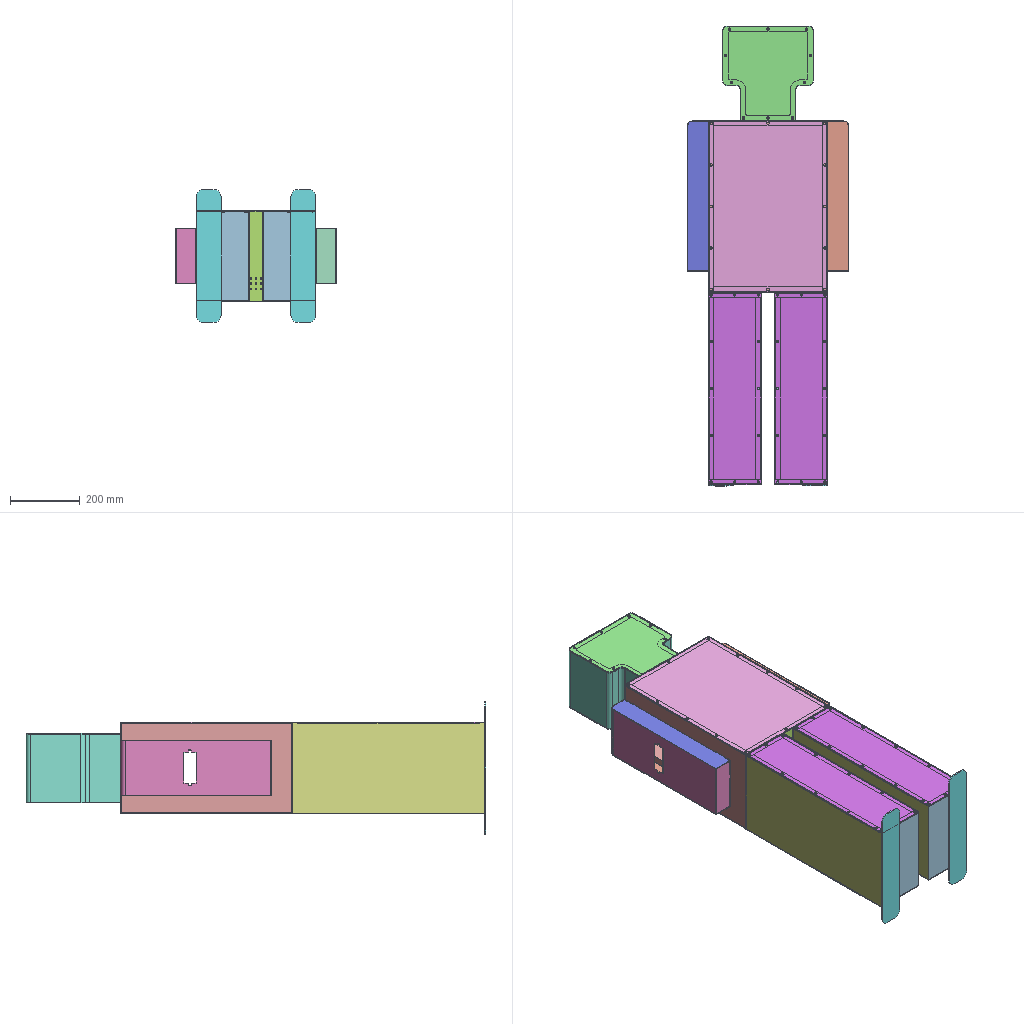Assembly | SolidWorks | 23 different items | 65 placed | box 460 x 1314 x 380 mm
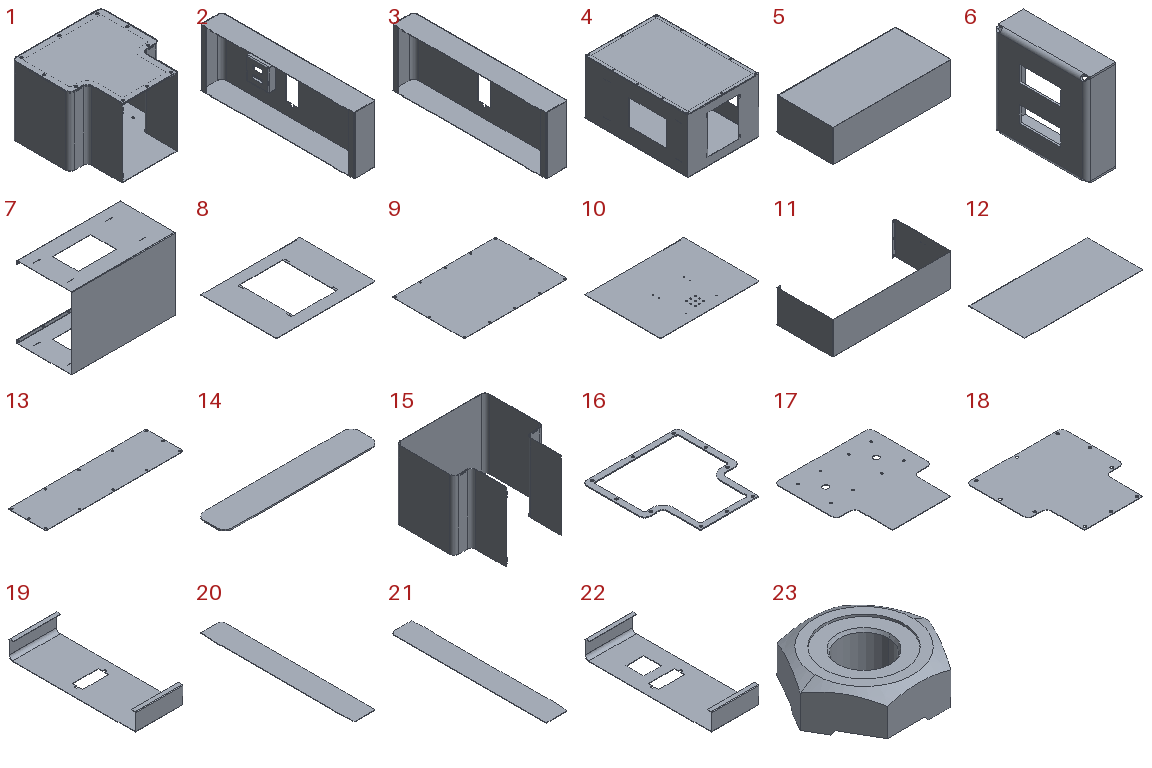Parts list (item | name | quantity | parent item | size | volume | features):
1 | (subassembly) | x1 | - | 260 x 272 x 200 mm | 384114 mm3 | -
2 | (subassembly) | x1 | - | 61.2 x 430 x 160 mm | 170255 mm3 | -
3 | (subassembly) | x1 | - | 61.2 x 430 x 160 mm | 165436 mm3 | -
4 | (subassembly) | x1 | - | 340 x 490 x 261.2 mm | 851284 mm3 | -
5 | (subassembly) | x2 | - | 550 x 261.2 x 150 mm | 653349 mm3 | features MirrorCompFeat 1, ReferencePattern 1
6 | - | x1 | in 2 | 20 x 62.4 x 62.4 mm | 9139 mm3 | features BaseBody 1
7 | - | x1 | in 4 | 487.6 x 260 x 340 mm | 463191 mm3 | features ICE 2, Cut 1, FlatPattern 1, MirrorPattern 1, SMBaseFlange 1, SheetMetal 1
8 | - | x1 | in 4 | 340 x 260 x 15 mm | 78192 mm3 | features Cut 2, EdgeFlange 1, FlatPattern 1, ICE 1, SMBaseFlange 1, SheetMetal 1
9 | - | x1 | in 4 | 490 x 340 x 1.2 mm | 199340 mm3 | features FlatPattern 1, SMBaseFlange 1, SheetMetal 1
10 | - | x1 | in 4 | 340 x 260 x 15 mm | 110561 mm3 | features ICE 2, EdgeFlange 1, FlatPattern 1, SMBaseFlange 1, SheetMetal 1
11 | - | x2 | in 5 | 550 x 260 x 150 mm | 196185 mm3 | features Cut 1, FlatPattern 1, ICE 1, SMBaseFlange 1, SheetMetal 1
12 | - | x4 | in 5 | 547.6 x 258.8 x 15 mm | 177930 mm3 | features EdgeFlange 1, FlatPattern 1, ICE 1, SMBaseFlange 1, SheetMetal 1
13 | - | x2 | in 5 | 550 x 150 x 1.2 mm | 98420 mm3 | features FlatPattern 1, SMBaseFlange 1, SheetMetal 1
14 | - | x2 | - | 380 x 70 x 3.2 mm | 84021 mm3 | features FlatPattern 1, SMBaseFlange 1, SheetMetal 1
15 | - | x1 | in 1 | 260 x 272 x 200 mm | 208024 mm3 | features ICE 2, SMBaseFlange 2, FlatPattern 1, MirrorPattern 1, SheetMetal 1
16 | - | x1 | in 1 | 257.6 x 269.6 x 2.3 mm | 32681 mm3 | features SMBaseFlange 2, FlatPattern 1, ICE 1, SheetMetal 1
17 | - | x1 | in 1 | 257.6 x 269.6 x 1.2 mm | 70428 mm3 | features HoleWzd 2, FlatPattern 1, SMBaseFlange 1, SheetMetal 1
18 | - | x1 | in 1 | 257.6 x 269.6 x 1.2 mm | 70578 mm3 | features FlatPattern 1, SMBaseFlange 1, SheetMetal 1
19 | - | x1 | in 3 | 160 x 430 x 60 mm | 105063 mm3 | features FlatPattern 1, ICE 1, SMBaseFlange 1, SheetMetal 1
20 | - | x2 | in 2, 3 | 60 x 427.6 x 1.2 mm | 30186 mm3 | features EdgeFlange 1, FlatPattern 1, SMBaseFlange 1, SheetMetal 1
21 | - | x2 | in 2, 3 | 60 x 427.6 x 1.2 mm | 30186 mm3 | features EdgeFlange 1, FlatPattern 1, SMBaseFlange 1, SheetMetal 1
22 | - | x1 | in 2 | 160 x 430 x 60 mm | 100743 mm3 | features FlatPattern 1, ICE 1, SMBaseFlange 1, SheetMetal 1
23 | - | x34 | in 1, 5 | 11.547 x 10 x 4 mm | 240.353 mm3 | features Cut 2, RevCut 2, Boss 1, Chamfer 1, CirPattern 1, Draft 1, Extrusion 1, LPattern 1, RefAxis 1
Mates (type | each side: item.copy, entity, surface, feature):
In the top assembly
Coincident | 8.1 face plane Base-Flange1 | 15.1 face plane Base-Flange1
DistanceDim | 7.1 face plane Base-Flange1 | 17.1 face plane Base-Flange1
DistanceDim | 15.1 face plane Base-Flange1 | 7.1 face plane Base-Flange1
Coincident | 10.1 face plane Base-Flange1 | 11.1 face plane Base-Flange1
Coincident | 7.1 face plane Base-Flange1 | 12.1 face plane Base-Flange1
Coincident | 7.1 face plane Base-Flange1 | 11.1 face plane Base-Flange1
Coincident | 10.1 face plane Base-Flange1 | 11.2 face plane Base-Flange1
Coincident | 7.1 face plane Base-Flange1 | 11.2 face plane Base-Flange1
Coincident | 7.1 face plane Base-Flange1 | 12.2 face plane Base-Flange1
Coincident | 7.1 face plane Base-Flange1 | 22.1 edge
Coincident | 8.1 face plane Base-Flange1 | 22.1 face plane Base-Flange1
DistanceDim | 7.1 face plane Base-Flange1 | 21.1 face plane Base-Flange1
Coincident | 7.1 face plane Base-Flange1 | 19.1 edge
Coincident | 8.1 face plane Base-Flange1 | 19.1 face plane Base-Flange1
DistanceDim | 7.1 face plane Base-Flange1 | 20.1 face plane Base-Flange1
Coincident | 11.2 face plane Base-Flange1 | 14.1 face plane Base-Flange1
Coincident | 12.2 face plane Base-Flange1 | 14.1 face plane Base-Flange1
DistanceDim | 11.2 face plane Base-Flange1 | 14.1 face plane Base-Flange1
In subassembly 2
InPlace | 22.2 face plane Base-Flange1 | 20.2 plane
InPlace | 22.2 face plane Base-Flange1 | 21.2 plane
Coincident | 22.2 face plane Base-Flange1 | 6.1 face plane Input1
Coincident | 22.2 face plane Cut-Extrude1 | 6.1 face plane Input1 | 2 times
In subassembly 3
InPlace | 19.2 face plane Base-Flange1 | 20.2 plane
InPlace | 19.2 face plane Base-Flange1 | 21.2 plane
In subassembly 5
InPlace | 11.3 face plane Base-Flange1 | 12.3 plane
InPlace | 12.3 face plane Edge-Flange1 | 13.1 plane
Concentric | 12.3 face cylinder Cut-Extrude1 | 23.1 face cylinder Cut-Extrude1
Coincident | 12.3 face plane Edge-Flange1 | 23.1 face plane BaseNut
Concentric | 12.3 face cylinder Cut-Extrude1 | 23.2 face cylinder Cut-Extrude1
Coincident | 12.3 face plane Edge-Flange1 | 23.2 face plane BaseNut
Concentric | 12.3 face cylinder Cut-Extrude1 | 23.3 face cylinder Cut-Extrude1
Coincident | 12.3 face plane Edge-Flange1 | 23.3 face plane BaseNut
Concentric | 12.4 face cylinder Cut-Extrude1 | 23.4 face cylinder Cut-Extrude1
Coincident | 12.4 face plane Edge-Flange1 | 23.4 face plane BaseNut
Concentric | 12.4 face cylinder Cut-Extrude1 | 23.5 face cylinder Cut-Extrude1
Coincident | 12.4 face plane Edge-Flange1 | 23.5 face plane BaseNut
Concentric | 12.4 face cylinder Cut-Extrude1 | 23.6 face cylinder Cut-Extrude1
Coincident | 12.4 face plane Edge-Flange1 | 23.6 face plane BaseNut
Concentric | 11.3 face cylinder Cut-Extrude1 | 23.7 face cylinder Cut-Extrude1
Coincident | 11.3 face plane Base-Flange1 | 23.7 face plane BaseNut
Concentric | 11.3 face cylinder Cut-Extrude1 | 23.8 face cylinder Cut-Extrude1
Coincident | 11.3 face plane Base-Flange1 | 23.8 face plane BaseNut
Concentric | 11.3 face cylinder Cut-Extrude1 | 23.9 face cylinder Cut-Extrude1
Coincident | 11.3 face plane Base-Flange1 | 23.9 face plane BaseNut
Concentric | 11.3 face cylinder Cut-Extrude1 | 23.10 face cylinder Cut-Extrude1
Coincident | 11.3 face plane Base-Flange1 | 23.10 face plane BaseNut
Concentric | 11.3 face cylinder Cut-Extrude1 | 23.11 face cylinder Cut-Extrude1
Coincident | 11.3 face plane Base-Flange1 | 23.11 face plane BaseNut
In subassembly 4
Coincident | 7.2 face plane Base-Flange1 | 8.2 face plane Base-Flange1 | 3 times
Coincident | 7.2 face plane Base-Flange1 | 10.2 face plane Base-Flange1 | 3 times
Coincident | 7.2 face plane Base-Flange1 | 9.1 face plane Base-Flange1 | 2 times
Coincident | 8.2 face plane Base-Flange1 | 9.1 face plane Base-Flange1
In subassembly 1
Coincident | 15.2 face plane Base-Flange1 | 17.2 face plane Base-Flange1 | 3 times
Coincident | 15.2 face plane Base-Flange1 | 16.1 face plane Base-Flange1 | 2 times
Coincident | 15.2 face plane Cut-Extrude2 | 16.1 face plane Base-Flange1
Coincident | 16.1 face plane Base-Flange1 | 18.1 face plane Base-Flange1
Coincident | 15.2 face plane Base-Flange1 | 18.1 face plane Base-Flange1 | 2 times
Concentric | 16.1 face cylinder Cut-Extrude1 | 23.1 face cylinder Cut-Extrude1
Coincident | 16.1 face plane Base-Flange1 | 23.1 face plane BaseNut
Concentric | 16.1 face cylinder Cut-Extrude1 | 23.2 face cylinder Cut-Extrude1
Coincident | 16.1 face plane Base-Flange1 | 23.2 face plane BaseNut
Concentric | 16.1 face cylinder Cut-Extrude1 | 23.3 face cylinder Cut-Extrude1
Coincident | 16.1 face plane Base-Flange1 | 23.3 face plane BaseNut
Concentric | 16.1 face cylinder Cut-Extrude1 | 23.4 face cylinder Cut-Extrude1
Coincident | 16.1 face plane Base-Flange1 | 23.4 face plane BaseNut
Concentric | 16.1 face cylinder Cut-Extrude1 | 23.5 face cylinder Cut-Extrude1
Coincident | 16.1 face plane Base-Flange1 | 23.5 face plane BaseNut
Concentric | 23.6 face cylinder Cut-Extrude1 | 16.1 face cylinder Cut-Extrude1
Coincident | 16.1 face plane Base-Flange1 | 23.6 face plane BaseNut
Concentric | 23.7 face cylinder Cut-Extrude1 | 16.1 face cylinder Cut-Extrude1
Coincident | 16.1 face plane Base-Flange1 | 23.7 face plane BaseNut
Concentric | 23.8 face cylinder Cut-Extrude1 | 16.1 face cylinder Cut-Extrude1
Coincident | 16.1 face plane Base-Flange1 | 23.8 face plane BaseNut
Concentric | 16.1 face cylinder Cut-Extrude1 | 23.12 face cylinder Cut-Extrude1
Coincident | 16.1 face plane Base-Flange1 | 23.12 face plane BaseNut
Concentric | 16.1 face cylinder Cut-Extrude1 | 23.9 face cylinder Cut-Extrude1
Coincident | 16.1 face plane Base-Flange1 | 23.9 face plane BaseNut